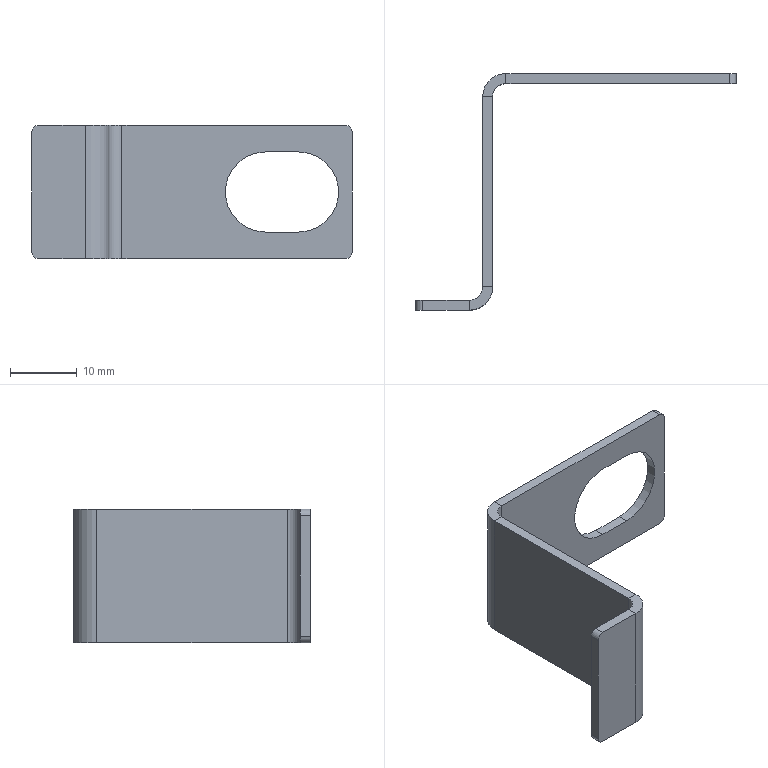Part | STEP file | 001-004-Feeding mechanism proximity switch mounting sheet metal | 1 solid | 30 faces | box 48 x 35.5 x 20 mm | volume 2128 mm3 | plane 20 | cylinder 10 | commonest cylinder face diameters 2 x4 4 x2 7 x2 12 x2